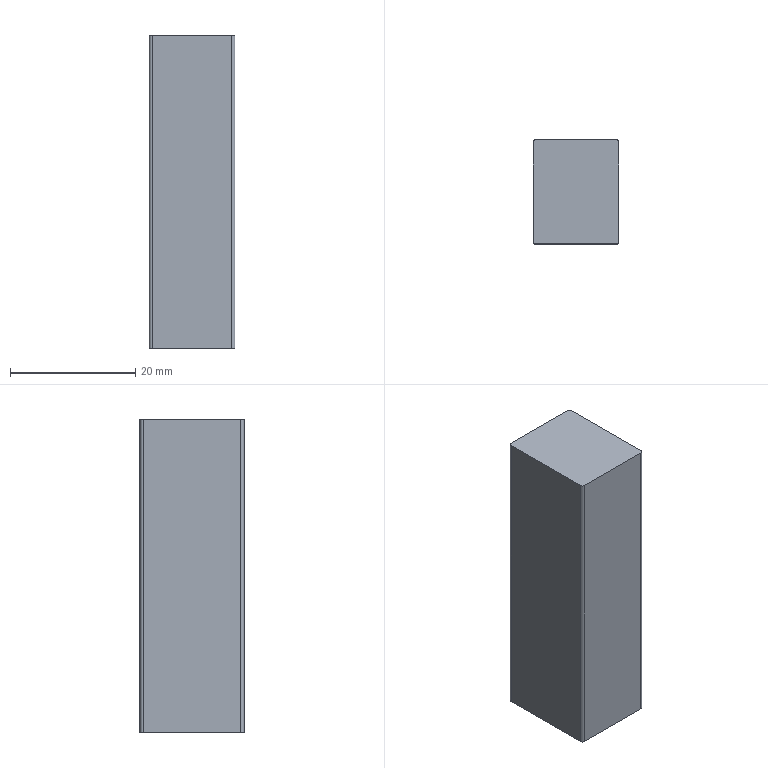Part | NX | features BREP 1 | 1 solid | 10 faces | box 13.7 x 16.6 x 50 mm | volume 11360 mm3 | plane 6 | cylinder 4 | commonest cylinder face diameters 1 x4
STEP:
#1=CARTESIAN_POINT('',(-6.35,8.3,-40.6));
#2=VERTEX_POINT('',#1);
#3=CARTESIAN_POINT('',(-6.85,7.8,-40.6));
#4=VERTEX_POINT('',#3);
#5=CARTESIAN_POINT('',(-6.35,7.8,-40.6));
#6=DIRECTION('',(0.,0.,1.));
#7=DIRECTION('',(1.,0.,0.));
#8=AXIS2_PLACEMENT_3D('',#5,#6,#7);
#9=CIRCLE('',#8,0.5);
#10=EDGE_CURVE('',#2,#4,#9,.T.);
#11=ORIENTED_EDGE('',*,*,#10,.F.);
#12=CARTESIAN_POINT('',(-6.35,8.3,-90.6));
#13=VERTEX_POINT('',#12);
#14=CARTESIAN_POINT('',(-6.35,8.3,-90.6));
#15=DIRECTION('',(0.,0.,1.));
#16=VECTOR('',#15,1000.);
#17=LINE('',#14,#16);
#18=EDGE_CURVE('',#13,#2,#17,.T.);
#19=ORIENTED_EDGE('',*,*,#18,.F.);
#20=CARTESIAN_POINT('',(-6.85,7.8,-90.6));
#21=VERTEX_POINT('',#20);
#22=CARTESIAN_POINT('',(-6.35,7.8,-90.6));
#23=DIRECTION('',(0.,0.,1.));
#24=DIRECTION('',(1.,0.,0.));
#25=AXIS2_PLACEMENT_3D('',#22,#23,#24);
#26=CIRCLE('',#25,0.5);
#27=EDGE_CURVE('',#13,#21,#26,.T.);
#28=ORIENTED_EDGE('',*,*,#27,.T.);
#29=CARTESIAN_POINT('',(-6.85,7.8,-90.6));
#30=DIRECTION('',(0.,0.,1.));
#31=VECTOR('',#30,1000.);
#32=LINE('',#29,#31);
#33=EDGE_CURVE('',#21,#4,#32,.T.);
#34=ORIENTED_EDGE('',*,*,#33,.T.);
#35=EDGE_LOOP('',(#11,#19,#28,#34));
#36=FACE_BOUND('',#35,.T.);
#37=CARTESIAN_POINT('',(-6.35,7.8,-90.6));
#38=DIRECTION('',(0.,0.,1.));
#39=DIRECTION('',(-1.,0.,0.));
#40=AXIS2_PLACEMENT_3D('',#37,#38,#39);
#41=CYLINDRICAL_SURFACE('',#40,0.5);
#42=ADVANCED_FACE('',(#36),#41,.T.);
#43=CARTESIAN_POINT('',(-6.85,-7.8,-40.6));
#44=VERTEX_POINT('',#43);
#45=CARTESIAN_POINT('',(-6.85,-7.8,-40.6));
#46=DIRECTION('',(0.,1.,0.));
#47=VECTOR('',#46,1000.);
#48=LINE('',#45,#47);
#49=EDGE_CURVE('',#44,#4,#48,.T.);
#50=ORIENTED_EDGE('',*,*,#49,.T.);
#51=ORIENTED_EDGE('',*,*,#33,.F.);
#52=CARTESIAN_POINT('',(-6.85,-7.8,-90.6));
#53=VERTEX_POINT('',#52);
#54=CARTESIAN_POINT('',(-6.85,-7.8,-90.6));
#55=DIRECTION('',(0.,1.,0.));
#56=VECTOR('',#55,1000.);
#57=LINE('',#54,#56);
#58=EDGE_CURVE('',#53,#21,#57,.T.);
#59=ORIENTED_EDGE('',*,*,#58,.F.);
#60=CARTESIAN_POINT('',(-6.85,-7.8,-90.6));
#61=DIRECTION('',(0.,0.,1.));
#62=VECTOR('',#61,1000.);
#63=LINE('',#60,#62);
#64=EDGE_CURVE('',#53,#44,#63,.T.);
#65=ORIENTED_EDGE('',*,*,#64,.T.);
#66=EDGE_LOOP('',(#50,#51,#59,#65));
#67=FACE_BOUND('',#66,.T.);
#68=CARTESIAN_POINT('',(-6.85,-7.8,-90.6));
#69=DIRECTION('',(1.,0.,0.));
#70=DIRECTION('',(0.,0.,1.));
#71=AXIS2_PLACEMENT_3D('',#68,#69,#70);
#72=PLANE('',#71);
#73=ADVANCED_FACE('',(#67),#72,.F.);
#74=CARTESIAN_POINT('',(-6.35,-8.3,-40.6));
#75=VERTEX_POINT('',#74);
#76=CARTESIAN_POINT('',(-6.35,-7.8,-40.6));
#77=DIRECTION('',(0.,0.,1.));
#78=DIRECTION('',(1.,0.,0.));
#79=AXIS2_PLACEMENT_3D('',#76,#77,#78);
#80=CIRCLE('',#79,0.5);
#81=EDGE_CURVE('',#44,#75,#80,.T.);
#82=ORIENTED_EDGE('',*,*,#81,.F.);
#83=ORIENTED_EDGE('',*,*,#64,.F.);
#84=CARTESIAN_POINT('',(-6.35,-8.3,-90.6));
#85=VERTEX_POINT('',#84);
#86=CARTESIAN_POINT('',(-6.35,-7.8,-90.6));
#87=DIRECTION('',(0.,0.,1.));
#88=DIRECTION('',(1.,0.,0.));
#89=AXIS2_PLACEMENT_3D('',#86,#87,#88);
#90=CIRCLE('',#89,0.5);
#91=EDGE_CURVE('',#53,#85,#90,.T.);
#92=ORIENTED_EDGE('',*,*,#91,.T.);
#93=CARTESIAN_POINT('',(-6.35,-8.3,-90.6));
#94=DIRECTION('',(0.,0.,1.));
#95=VECTOR('',#94,1000.);
#96=LINE('',#93,#95);
#97=EDGE_CURVE('',#85,#75,#96,.T.);
#98=ORIENTED_EDGE('',*,*,#97,.T.);
#99=EDGE_LOOP('',(#82,#83,#92,#98));
#100=FACE_BOUND('',#99,.T.);
#101=CARTESIAN_POINT('',(-6.35,-7.8,-90.6));
#102=DIRECTION('',(0.,0.,1.));
#103=DIRECTION('',(-1.,0.,0.));
#104=AXIS2_PLACEMENT_3D('',#101,#102,#103);
#105=CYLINDRICAL_SURFACE('',#104,0.5);
#106=ADVANCED_FACE('',(#100),#105,.T.);
#107=CARTESIAN_POINT('',(6.35,-8.3,-40.6));
#108=VERTEX_POINT('',#107);
#109=CARTESIAN_POINT('',(6.35,-8.3,-40.6));
#110=DIRECTION('',(-1.,0.,0.));
#111=VECTOR('',#110,1000.);
#112=LINE('',#109,#111);
#113=EDGE_CURVE('',#108,#75,#112,.T.);
#114=ORIENTED_EDGE('',*,*,#113,.T.);
#115=ORIENTED_EDGE('',*,*,#97,.F.);
#116=CARTESIAN_POINT('',(6.35,-8.3,-90.6));
#117=VERTEX_POINT('',#116);
#118=CARTESIAN_POINT('',(6.35,-8.3,-90.6));
#119=DIRECTION('',(-1.,0.,0.));
#120=VECTOR('',#119,1000.);
#121=LINE('',#118,#120);
#122=EDGE_CURVE('',#117,#85,#121,.T.);
#123=ORIENTED_EDGE('',*,*,#122,.F.);
#124=CARTESIAN_POINT('',(6.35,-8.3,-90.6));
#125=DIRECTION('',(0.,0.,1.));
#126=VECTOR('',#125,1000.);
#127=LINE('',#124,#126);
#128=EDGE_CURVE('',#117,#108,#127,.T.);
#129=ORIENTED_EDGE('',*,*,#128,.T.);
#130=EDGE_LOOP('',(#114,#115,#123,#129));
#131=FACE_BOUND('',#130,.T.);
#132=CARTESIAN_POINT('',(6.35,-8.3,-90.6));
#133=DIRECTION('',(0.,1.,0.));
#134=DIRECTION('',(0.,0.,-1.));
#135=AXIS2_PLACEMENT_3D('',#132,#133,#134);
#136=PLANE('',#135);
#137=ADVANCED_FACE('',(#131),#136,.F.);
#138=CARTESIAN_POINT('',(6.85,-7.8,-40.6));
#139=VERTEX_POINT('',#138);
#140=CARTESIAN_POINT('',(6.35,-7.8,-40.6));
#141=DIRECTION('',(0.,0.,1.));
#142=DIRECTION('',(1.,0.,0.));
#143=AXIS2_PLACEMENT_3D('',#140,#141,#142);
#144=CIRCLE('',#143,0.5);
#145=EDGE_CURVE('',#108,#139,#144,.T.);
#146=ORIENTED_EDGE('',*,*,#145,.F.);
#147=ORIENTED_EDGE('',*,*,#128,.F.);
#148=CARTESIAN_POINT('',(6.85,-7.8,-90.6));
#149=VERTEX_POINT('',#148);
#150=CARTESIAN_POINT('',(6.35,-7.8,-90.6));
#151=DIRECTION('',(0.,0.,1.));
#152=DIRECTION('',(1.,0.,0.));
#153=AXIS2_PLACEMENT_3D('',#150,#151,#152);
#154=CIRCLE('',#153,0.5);
#155=EDGE_CURVE('',#117,#149,#154,.T.);
#156=ORIENTED_EDGE('',*,*,#155,.T.);
#157=CARTESIAN_POINT('',(6.85,-7.8,-90.6));
#158=DIRECTION('',(0.,0.,1.));
#159=VECTOR('',#158,1000.);
#160=LINE('',#157,#159);
#161=EDGE_CURVE('',#149,#139,#160,.T.);
#162=ORIENTED_EDGE('',*,*,#161,.T.);
#163=EDGE_LOOP('',(#146,#147,#156,#162));
#164=FACE_BOUND('',#163,.T.);
#165=CARTESIAN_POINT('',(6.35,-7.8,-90.6));
#166=DIRECTION('',(0.,0.,1.));
#167=DIRECTION('',(-1.,0.,0.));
#168=AXIS2_PLACEMENT_3D('',#165,#166,#167);
#169=CYLINDRICAL_SURFACE('',#168,0.5);
#170=ADVANCED_FACE('',(#164),#169,.T.);
#171=CARTESIAN_POINT('',(6.85,7.8,-40.6));
#172=VERTEX_POINT('',#171);
#173=CARTESIAN_POINT('',(6.85,7.8,-40.6));
#174=DIRECTION('',(0.,-1.,0.));
#175=VECTOR('',#174,1000.);
#176=LINE('',#173,#175);
#177=EDGE_CURVE('',#172,#139,#176,.T.);
#178=ORIENTED_EDGE('',*,*,#177,.T.);
#179=ORIENTED_EDGE('',*,*,#161,.F.);
#180=CARTESIAN_POINT('',(6.85,7.8,-90.6));
#181=VERTEX_POINT('',#180);
#182=CARTESIAN_POINT('',(6.85,7.8,-90.6));
#183=DIRECTION('',(0.,-1.,0.));
#184=VECTOR('',#183,1000.);
#185=LINE('',#182,#184);
#186=EDGE_CURVE('',#181,#149,#185,.T.);
#187=ORIENTED_EDGE('',*,*,#186,.F.);
#188=CARTESIAN_POINT('',(6.85,7.8,-90.6));
#189=DIRECTION('',(0.,0.,1.));
#190=VECTOR('',#189,1000.);
#191=LINE('',#188,#190);
#192=EDGE_CURVE('',#181,#172,#191,.T.);
#193=ORIENTED_EDGE('',*,*,#192,.T.);
#194=EDGE_LOOP('',(#178,#179,#187,#193));
#195=FACE_BOUND('',#194,.T.);
#196=CARTESIAN_POINT('',(6.85,7.8,-90.6));
#197=DIRECTION('',(-1.,0.,0.));
#198=DIRECTION('',(0.,1.,0.));
#199=AXIS2_PLACEMENT_3D('',#196,#197,#198);
#200=PLANE('',#199);
#201=ADVANCED_FACE('',(#195),#200,.F.);
#202=CARTESIAN_POINT('',(6.35,8.3,-40.6));
#203=VERTEX_POINT('',#202);
#204=CARTESIAN_POINT('',(6.35,7.8,-40.6));
#205=DIRECTION('',(0.,0.,1.));
#206=DIRECTION('',(1.,0.,0.));
#207=AXIS2_PLACEMENT_3D('',#204,#205,#206);
#208=CIRCLE('',#207,0.5);
#209=EDGE_CURVE('',#172,#203,#208,.T.);
#210=ORIENTED_EDGE('',*,*,#209,.F.);
#211=ORIENTED_EDGE('',*,*,#192,.F.);
#212=CARTESIAN_POINT('',(6.35,8.3,-90.6));
#213=VERTEX_POINT('',#212);
#214=CARTESIAN_POINT('',(6.35,7.8,-90.6));
#215=DIRECTION('',(0.,0.,1.));
#216=DIRECTION('',(1.,0.,0.));
#217=AXIS2_PLACEMENT_3D('',#214,#215,#216);
#218=CIRCLE('',#217,0.5);
#219=EDGE_CURVE('',#181,#213,#218,.T.);
#220=ORIENTED_EDGE('',*,*,#219,.T.);
#221=CARTESIAN_POINT('',(6.35,8.3,-90.6));
#222=DIRECTION('',(0.,0.,1.));
#223=VECTOR('',#222,1000.);
#224=LINE('',#221,#223);
#225=EDGE_CURVE('',#213,#203,#224,.T.);
#226=ORIENTED_EDGE('',*,*,#225,.T.);
#227=EDGE_LOOP('',(#210,#211,#220,#226));
#228=FACE_BOUND('',#227,.T.);
#229=CARTESIAN_POINT('',(6.35,7.8,-90.6));
#230=DIRECTION('',(0.,0.,1.));
#231=DIRECTION('',(-1.,0.,0.));
#232=AXIS2_PLACEMENT_3D('',#229,#230,#231);
#233=CYLINDRICAL_SURFACE('',#232,0.5);
#234=ADVANCED_FACE('',(#228),#233,.T.);
#235=CARTESIAN_POINT('',(-6.35,8.3,-40.6));
#236=DIRECTION('',(1.,0.,0.));
#237=VECTOR('',#236,1000.);
#238=LINE('',#235,#237);
#239=EDGE_CURVE('',#2,#203,#238,.T.);
#240=ORIENTED_EDGE('',*,*,#239,.T.);
#241=ORIENTED_EDGE('',*,*,#225,.F.);
#242=CARTESIAN_POINT('',(-6.35,8.3,-90.6));
#243=DIRECTION('',(1.,0.,0.));
#244=VECTOR('',#243,1000.);
#245=LINE('',#242,#244);
#246=EDGE_CURVE('',#13,#213,#245,.T.);
#247=ORIENTED_EDGE('',*,*,#246,.F.);
#248=ORIENTED_EDGE('',*,*,#18,.T.);
#249=EDGE_LOOP('',(#240,#241,#247,#248));
#250=FACE_BOUND('',#249,.T.);
#251=CARTESIAN_POINT('',(-6.35,8.3,-90.6));
#252=DIRECTION('',(0.,-1.,0.));
#253=DIRECTION('',(-1.,0.,0.));
#254=AXIS2_PLACEMENT_3D('',#251,#252,#253);
#255=PLANE('',#254);
#256=ADVANCED_FACE('',(#250),#255,.F.);
#257=ORIENTED_EDGE('',*,*,#27,.F.);
#258=ORIENTED_EDGE('',*,*,#246,.T.);
#259=ORIENTED_EDGE('',*,*,#219,.F.);
#260=ORIENTED_EDGE('',*,*,#186,.T.);
#261=ORIENTED_EDGE('',*,*,#155,.F.);
#262=ORIENTED_EDGE('',*,*,#122,.T.);
#263=ORIENTED_EDGE('',*,*,#91,.F.);
#264=ORIENTED_EDGE('',*,*,#58,.T.);
#265=EDGE_LOOP('',(#257,#258,#259,#260,#261,#262,#263,#264));
#266=FACE_BOUND('',#265,.T.);
#267=CARTESIAN_POINT('',(-6.35,7.8,-90.6));
#268=DIRECTION('',(0.,0.,1.));
#269=DIRECTION('',(-1.,0.,0.));
#270=AXIS2_PLACEMENT_3D('',#267,#268,#269);
#271=PLANE('',#270);
#272=ADVANCED_FACE('',(#266),#271,.F.);
#273=ORIENTED_EDGE('',*,*,#10,.T.);
#274=ORIENTED_EDGE('',*,*,#49,.F.);
#275=ORIENTED_EDGE('',*,*,#81,.T.);
#276=ORIENTED_EDGE('',*,*,#113,.F.);
#277=ORIENTED_EDGE('',*,*,#145,.T.);
#278=ORIENTED_EDGE('',*,*,#177,.F.);
#279=ORIENTED_EDGE('',*,*,#209,.T.);
#280=ORIENTED_EDGE('',*,*,#239,.F.);
#281=EDGE_LOOP('',(#273,#274,#275,#276,#277,#278,#279,#280));
#282=FACE_BOUND('',#281,.T.);
#283=CARTESIAN_POINT('',(-6.35,7.8,-40.6));
#284=DIRECTION('',(0.,0.,1.));
#285=DIRECTION('',(-1.,0.,0.));
#286=AXIS2_PLACEMENT_3D('',#283,#284,#285);
#287=PLANE('',#286);
#288=ADVANCED_FACE('',(#282),#287,.T.);
#289=CLOSED_SHELL('',(#42,#73,#106,#137,#170,#201,#234,#256,#272,#288));
#290=MANIFOLD_SOLID_BREP('',#289);
#291=(LENGTH_UNIT()NAMED_UNIT(*)SI_UNIT(.MILLI.,.METRE.));
#292=UNCERTAINTY_MEASURE_WITH_UNIT(LENGTH_MEASURE(0.00001),#291,'','');
#293=(NAMED_UNIT(*)PLANE_ANGLE_UNIT()SI_UNIT($,.RADIAN.));
#294=(NAMED_UNIT(*)SI_UNIT($,.STERADIAN.)SOLID_ANGLE_UNIT());
#295=(GEOMETRIC_REPRESENTATION_CONTEXT(3)GLOBAL_UNCERTAINTY_ASSIGNED_CONTEXT((#292))GLOBAL_UNIT_ASSIGNED_CONTEXT((#291,#293,#294))REPRESENTATION_CONTEXT('',''));
#296=ADVANCED_BREP_SHAPE_REPRESENTATION('',(#290),#295);